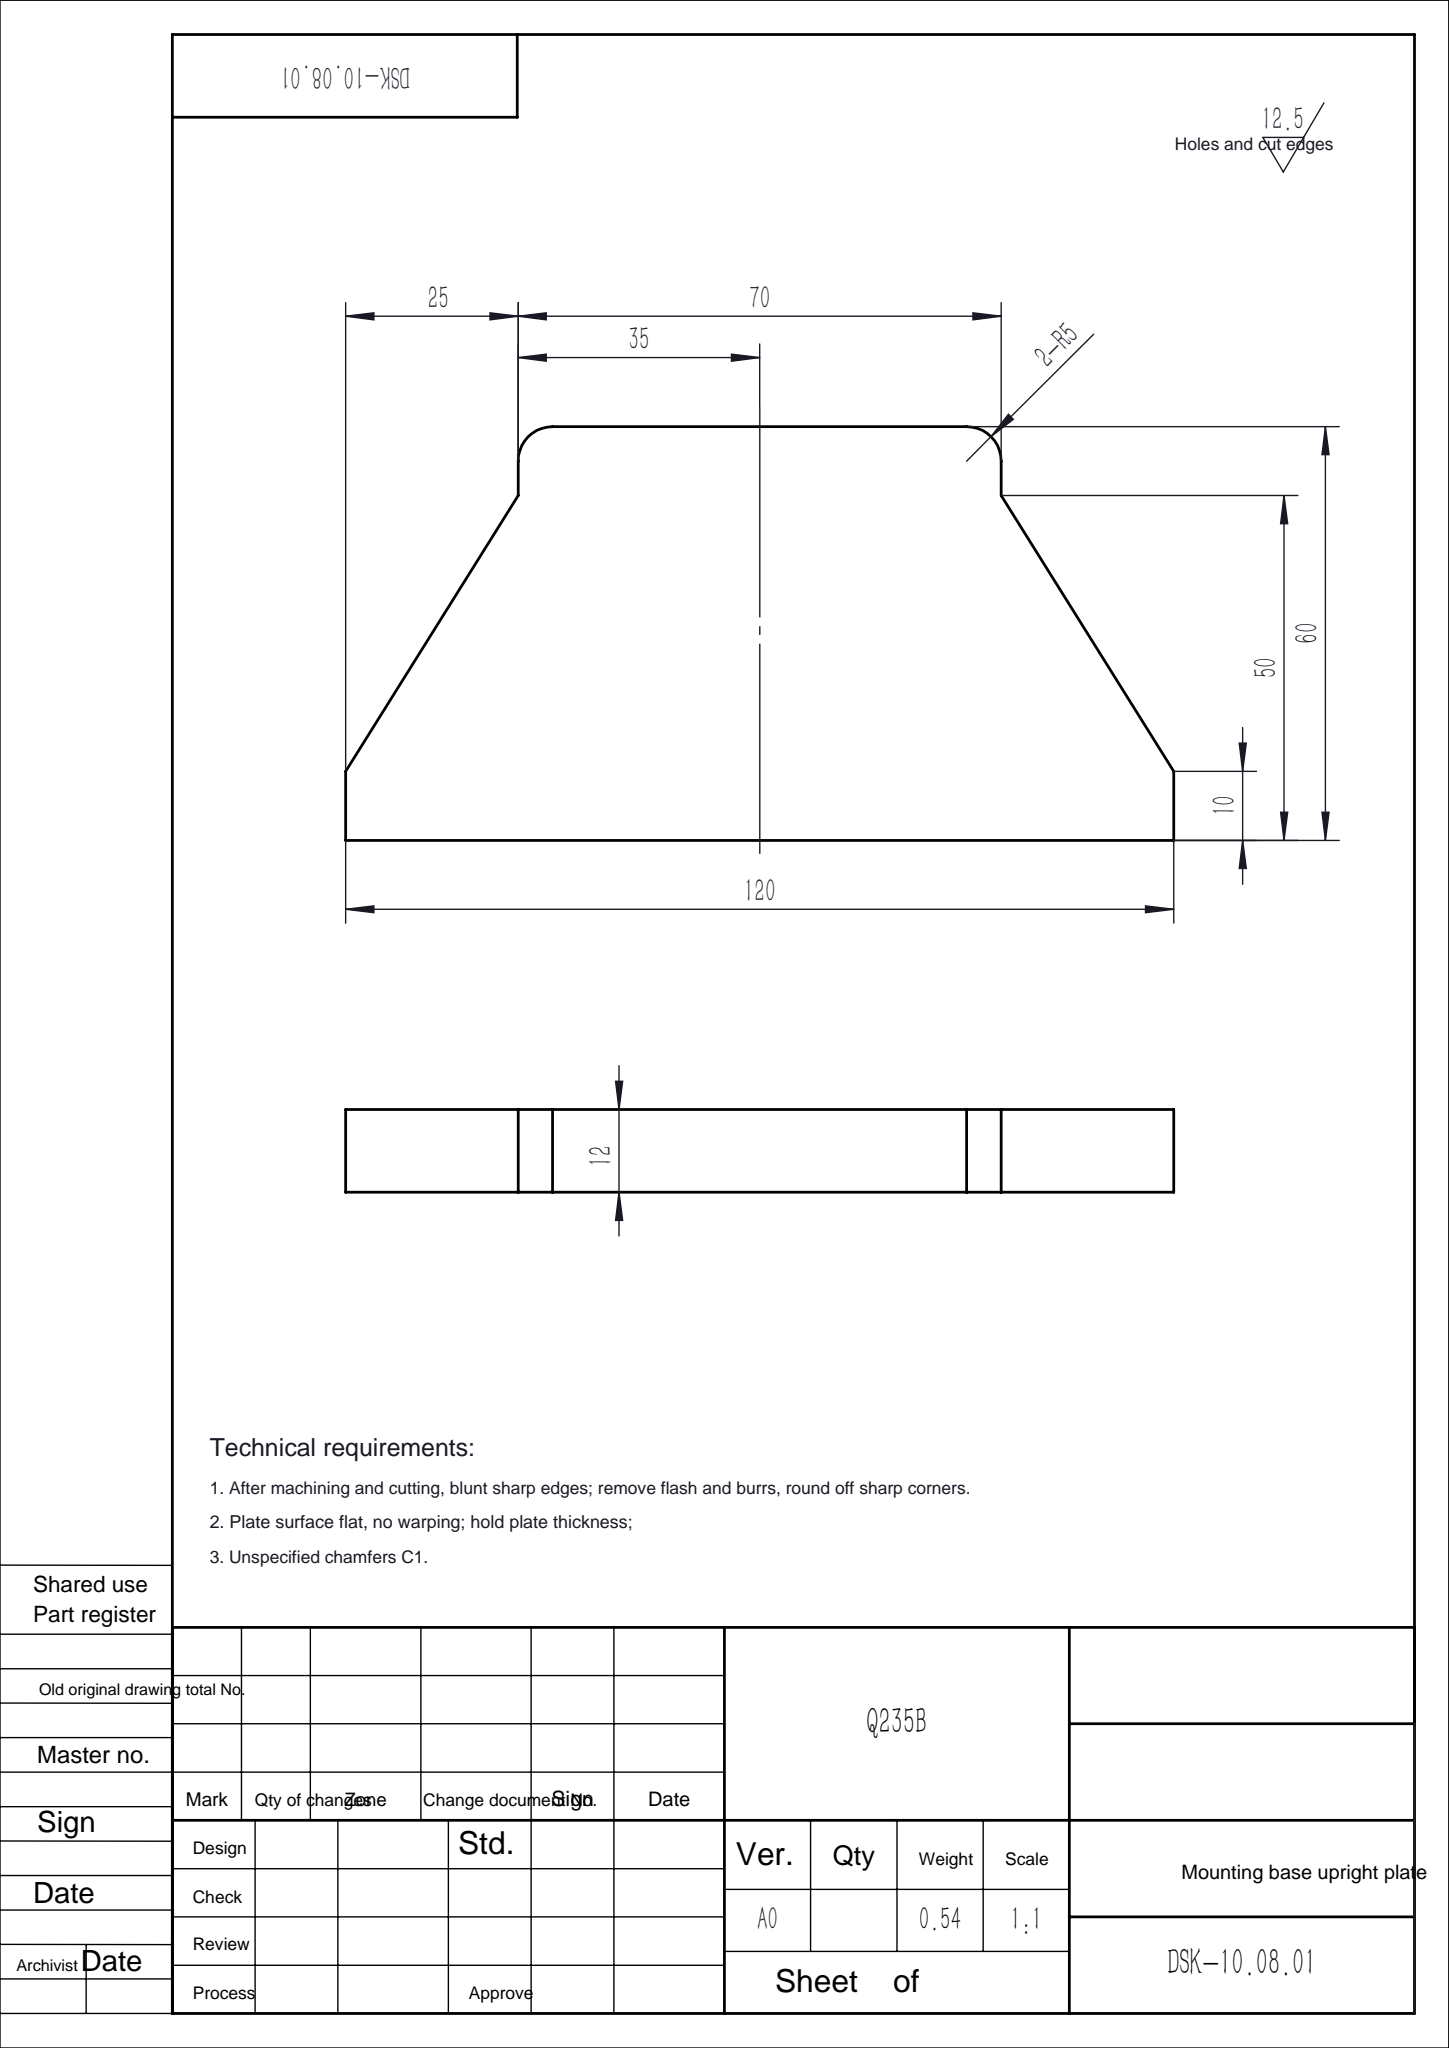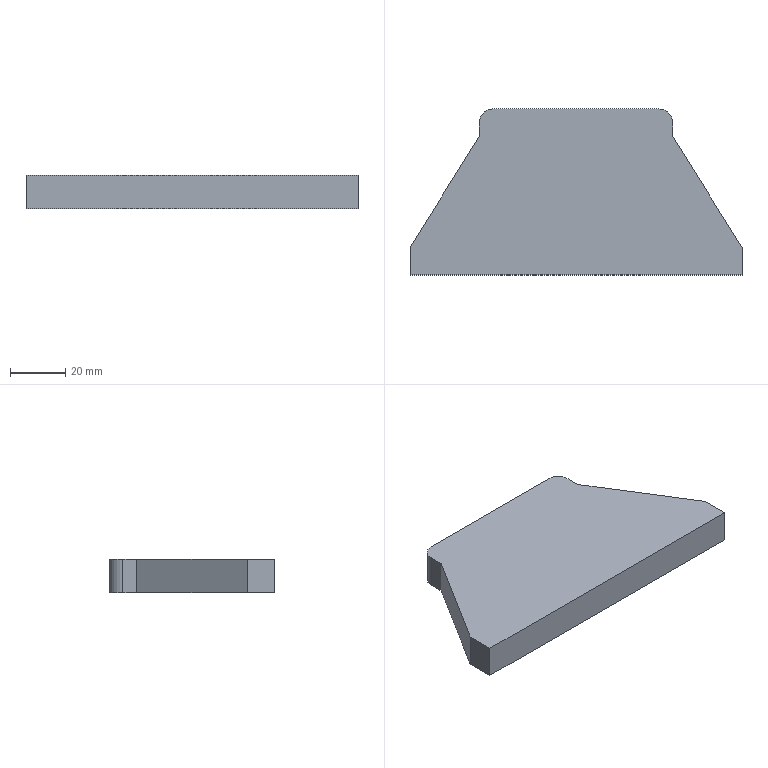Part | SolidWorks | features Extrusion 1, Fillet 1 | 1 solid | 12 faces | box 120 x 60 x 12 mm | volume 68271 mm3 | plane 10 | cylinder 2 | commonest cylinder face diameters 10 x2
STEP:
#1=CARTESIAN_POINT('',(60.,0.,-6.));
#2=VERTEX_POINT('',#1);
#3=CARTESIAN_POINT('',(60.,10.,-6.));
#4=VERTEX_POINT('',#3);
#5=CARTESIAN_POINT('',(60.,0.,-6.));
#6=DIRECTION('',(0.,1.,0.));
#7=VECTOR('',#6,1000.);
#8=LINE('',#5,#7);
#9=EDGE_CURVE('',#2,#4,#8,.T.);
#10=ORIENTED_EDGE('',*,*,#9,.T.);
#11=CARTESIAN_POINT('',(60.,10.,6.));
#12=VERTEX_POINT('',#11);
#13=CARTESIAN_POINT('',(60.,10.,6.));
#14=DIRECTION('',(0.,0.,-1.));
#15=VECTOR('',#14,1000.);
#16=LINE('',#13,#15);
#17=EDGE_CURVE('',#12,#4,#16,.T.);
#18=ORIENTED_EDGE('',*,*,#17,.F.);
#19=CARTESIAN_POINT('',(60.,0.,6.));
#20=VERTEX_POINT('',#19);
#21=CARTESIAN_POINT('',(60.,0.,6.));
#22=DIRECTION('',(0.,1.,0.));
#23=VECTOR('',#22,1000.);
#24=LINE('',#21,#23);
#25=EDGE_CURVE('',#20,#12,#24,.T.);
#26=ORIENTED_EDGE('',*,*,#25,.F.);
#27=CARTESIAN_POINT('',(60.,0.,6.));
#28=DIRECTION('',(0.,0.,-1.));
#29=VECTOR('',#28,1000.);
#30=LINE('',#27,#29);
#31=EDGE_CURVE('',#20,#2,#30,.T.);
#32=ORIENTED_EDGE('',*,*,#31,.T.);
#33=EDGE_LOOP('',(#10,#18,#26,#32));
#34=FACE_OUTER_BOUND('',#33,.T.);
#35=CARTESIAN_POINT('',(60.,0.,6.));
#36=DIRECTION('',(-1.,0.,0.));
#37=DIRECTION('',(0.,0.,1.));
#38=AXIS2_PLACEMENT_3D('',#35,#36,#37);
#39=PLANE('',#38);
#40=ADVANCED_FACE('',(#34),#39,.F.);
#41=CARTESIAN_POINT('',(35.,50.,-6.));
#42=VERTEX_POINT('',#41);
#43=CARTESIAN_POINT('',(60.,10.,-6.));
#44=DIRECTION('',(-0.53,0.848,0.));
#45=VECTOR('',#44,1000.);
#46=LINE('',#43,#45);
#47=EDGE_CURVE('',#4,#42,#46,.T.);
#48=ORIENTED_EDGE('',*,*,#47,.T.);
#49=CARTESIAN_POINT('',(35.,50.,6.));
#50=VERTEX_POINT('',#49);
#51=CARTESIAN_POINT('',(35.,50.,6.));
#52=DIRECTION('',(0.,0.,-1.));
#53=VECTOR('',#52,1000.);
#54=LINE('',#51,#53);
#55=EDGE_CURVE('',#50,#42,#54,.T.);
#56=ORIENTED_EDGE('',*,*,#55,.F.);
#57=CARTESIAN_POINT('',(60.,10.,6.));
#58=DIRECTION('',(-0.53,0.848,0.));
#59=VECTOR('',#58,1000.);
#60=LINE('',#57,#59);
#61=EDGE_CURVE('',#12,#50,#60,.T.);
#62=ORIENTED_EDGE('',*,*,#61,.F.);
#63=ORIENTED_EDGE('',*,*,#17,.T.);
#64=EDGE_LOOP('',(#48,#56,#62,#63));
#65=FACE_OUTER_BOUND('',#64,.T.);
#66=CARTESIAN_POINT('',(60.,10.,6.));
#67=DIRECTION('',(-0.848,-0.53,0.));
#68=DIRECTION('',(0.53,-0.848,0.));
#69=AXIS2_PLACEMENT_3D('',#66,#67,#68);
#70=PLANE('',#69);
#71=ADVANCED_FACE('',(#65),#70,.F.);
#72=CARTESIAN_POINT('',(35.,55.,-6.));
#73=VERTEX_POINT('',#72);
#74=CARTESIAN_POINT('',(35.,50.,-6.));
#75=DIRECTION('',(0.,1.,0.));
#76=VECTOR('',#75,1000.);
#77=LINE('',#74,#76);
#78=EDGE_CURVE('',#42,#73,#77,.T.);
#79=ORIENTED_EDGE('',*,*,#78,.T.);
#80=CARTESIAN_POINT('',(35.,55.,6.));
#81=VERTEX_POINT('',#80);
#82=CARTESIAN_POINT('',(35.,55.,6.));
#83=DIRECTION('',(0.,0.,1.));
#84=VECTOR('',#83,1000.);
#85=LINE('',#82,#84);
#86=EDGE_CURVE('',#73,#81,#85,.T.);
#87=ORIENTED_EDGE('',*,*,#86,.T.);
#88=CARTESIAN_POINT('',(35.,50.,6.));
#89=DIRECTION('',(0.,1.,0.));
#90=VECTOR('',#89,1000.);
#91=LINE('',#88,#90);
#92=EDGE_CURVE('',#50,#81,#91,.T.);
#93=ORIENTED_EDGE('',*,*,#92,.F.);
#94=ORIENTED_EDGE('',*,*,#55,.T.);
#95=EDGE_LOOP('',(#79,#87,#93,#94));
#96=FACE_OUTER_BOUND('',#95,.T.);
#97=CARTESIAN_POINT('',(35.,50.,6.));
#98=DIRECTION('',(-1.,0.,0.));
#99=DIRECTION('',(0.,0.,1.));
#100=AXIS2_PLACEMENT_3D('',#97,#98,#99);
#101=PLANE('',#100);
#102=ADVANCED_FACE('',(#96),#101,.F.);
#103=CARTESIAN_POINT('',(30.,60.,6.));
#104=VERTEX_POINT('',#103);
#105=CARTESIAN_POINT('',(-30.,60.,6.));
#106=VERTEX_POINT('',#105);
#107=CARTESIAN_POINT('',(35.,60.,6.));
#108=DIRECTION('',(-1.,0.,0.));
#109=VECTOR('',#108,1000.);
#110=LINE('',#107,#109);
#111=EDGE_CURVE('',#104,#106,#110,.T.);
#112=ORIENTED_EDGE('',*,*,#111,.F.);
#113=CARTESIAN_POINT('',(30.,60.,-6.));
#114=VERTEX_POINT('',#113);
#115=CARTESIAN_POINT('',(30.,60.,6.));
#116=DIRECTION('',(0.,0.,-1.));
#117=VECTOR('',#116,1000.);
#118=LINE('',#115,#117);
#119=EDGE_CURVE('',#104,#114,#118,.T.);
#120=ORIENTED_EDGE('',*,*,#119,.T.);
#121=CARTESIAN_POINT('',(-30.,60.,-6.));
#122=VERTEX_POINT('',#121);
#123=CARTESIAN_POINT('',(35.,60.,-6.));
#124=DIRECTION('',(-1.,0.,0.));
#125=VECTOR('',#124,1000.);
#126=LINE('',#123,#125);
#127=EDGE_CURVE('',#114,#122,#126,.T.);
#128=ORIENTED_EDGE('',*,*,#127,.T.);
#129=CARTESIAN_POINT('',(-30.,60.,6.));
#130=DIRECTION('',(0.,0.,1.));
#131=VECTOR('',#130,1000.);
#132=LINE('',#129,#131);
#133=EDGE_CURVE('',#122,#106,#132,.T.);
#134=ORIENTED_EDGE('',*,*,#133,.T.);
#135=EDGE_LOOP('',(#112,#120,#128,#134));
#136=FACE_OUTER_BOUND('',#135,.T.);
#137=CARTESIAN_POINT('',(35.,60.,6.));
#138=DIRECTION('',(0.,-1.,0.));
#139=DIRECTION('',(1.,0.,0.));
#140=AXIS2_PLACEMENT_3D('',#137,#138,#139);
#141=PLANE('',#140);
#142=ADVANCED_FACE('',(#136),#141,.F.);
#143=CARTESIAN_POINT('',(-35.,55.,6.));
#144=VERTEX_POINT('',#143);
#145=CARTESIAN_POINT('',(-35.,50.,6.));
#146=VERTEX_POINT('',#145);
#147=CARTESIAN_POINT('',(-35.,50.,6.));
#148=DIRECTION('',(0.,-1.,0.));
#149=VECTOR('',#148,1000.);
#150=LINE('',#147,#149);
#151=EDGE_CURVE('',#144,#146,#150,.T.);
#152=ORIENTED_EDGE('',*,*,#151,.F.);
#153=CARTESIAN_POINT('',(-35.,55.,-6.));
#154=VERTEX_POINT('',#153);
#155=CARTESIAN_POINT('',(-35.,55.,6.));
#156=DIRECTION('',(0.,0.,-1.));
#157=VECTOR('',#156,1000.);
#158=LINE('',#155,#157);
#159=EDGE_CURVE('',#144,#154,#158,.T.);
#160=ORIENTED_EDGE('',*,*,#159,.T.);
#161=CARTESIAN_POINT('',(-35.,50.,-6.));
#162=VERTEX_POINT('',#161);
#163=CARTESIAN_POINT('',(-35.,50.,-6.));
#164=DIRECTION('',(0.,-1.,0.));
#165=VECTOR('',#164,1000.);
#166=LINE('',#163,#165);
#167=EDGE_CURVE('',#154,#162,#166,.T.);
#168=ORIENTED_EDGE('',*,*,#167,.T.);
#169=CARTESIAN_POINT('',(-35.,50.,6.));
#170=DIRECTION('',(0.,0.,-1.));
#171=VECTOR('',#170,1000.);
#172=LINE('',#169,#171);
#173=EDGE_CURVE('',#146,#162,#172,.T.);
#174=ORIENTED_EDGE('',*,*,#173,.F.);
#175=EDGE_LOOP('',(#152,#160,#168,#174));
#176=FACE_OUTER_BOUND('',#175,.T.);
#177=CARTESIAN_POINT('',(-35.,50.,6.));
#178=DIRECTION('',(1.,0.,0.));
#179=DIRECTION('',(0.,0.,-1.));
#180=AXIS2_PLACEMENT_3D('',#177,#178,#179);
#181=PLANE('',#180);
#182=ADVANCED_FACE('',(#176),#181,.F.);
#183=CARTESIAN_POINT('',(-60.,10.,-6.));
#184=VERTEX_POINT('',#183);
#185=CARTESIAN_POINT('',(-60.,10.,-6.));
#186=DIRECTION('',(-0.53,-0.848,0.));
#187=VECTOR('',#186,1000.);
#188=LINE('',#185,#187);
#189=EDGE_CURVE('',#162,#184,#188,.T.);
#190=ORIENTED_EDGE('',*,*,#189,.T.);
#191=CARTESIAN_POINT('',(-60.,10.,6.));
#192=VERTEX_POINT('',#191);
#193=CARTESIAN_POINT('',(-60.,10.,6.));
#194=DIRECTION('',(0.,0.,-1.));
#195=VECTOR('',#194,1000.);
#196=LINE('',#193,#195);
#197=EDGE_CURVE('',#192,#184,#196,.T.);
#198=ORIENTED_EDGE('',*,*,#197,.F.);
#199=CARTESIAN_POINT('',(-60.,10.,6.));
#200=DIRECTION('',(-0.53,-0.848,0.));
#201=VECTOR('',#200,1000.);
#202=LINE('',#199,#201);
#203=EDGE_CURVE('',#146,#192,#202,.T.);
#204=ORIENTED_EDGE('',*,*,#203,.F.);
#205=ORIENTED_EDGE('',*,*,#173,.T.);
#206=EDGE_LOOP('',(#190,#198,#204,#205));
#207=FACE_OUTER_BOUND('',#206,.T.);
#208=CARTESIAN_POINT('',(-60.,10.,6.));
#209=DIRECTION('',(0.848,-0.53,0.));
#210=DIRECTION('',(0.53,0.848,0.));
#211=AXIS2_PLACEMENT_3D('',#208,#209,#210);
#212=PLANE('',#211);
#213=ADVANCED_FACE('',(#207),#212,.F.);
#214=CARTESIAN_POINT('',(-60.,0.,-6.));
#215=VERTEX_POINT('',#214);
#216=CARTESIAN_POINT('',(-60.,0.,-6.));
#217=DIRECTION('',(0.,-1.,0.));
#218=VECTOR('',#217,1000.);
#219=LINE('',#216,#218);
#220=EDGE_CURVE('',#184,#215,#219,.T.);
#221=ORIENTED_EDGE('',*,*,#220,.T.);
#222=CARTESIAN_POINT('',(-60.,0.,6.));
#223=VERTEX_POINT('',#222);
#224=CARTESIAN_POINT('',(-60.,0.,6.));
#225=DIRECTION('',(0.,0.,-1.));
#226=VECTOR('',#225,1000.);
#227=LINE('',#224,#226);
#228=EDGE_CURVE('',#223,#215,#227,.T.);
#229=ORIENTED_EDGE('',*,*,#228,.F.);
#230=CARTESIAN_POINT('',(-60.,0.,6.));
#231=DIRECTION('',(0.,-1.,0.));
#232=VECTOR('',#231,1000.);
#233=LINE('',#230,#232);
#234=EDGE_CURVE('',#192,#223,#233,.T.);
#235=ORIENTED_EDGE('',*,*,#234,.F.);
#236=ORIENTED_EDGE('',*,*,#197,.T.);
#237=EDGE_LOOP('',(#221,#229,#235,#236));
#238=FACE_OUTER_BOUND('',#237,.T.);
#239=CARTESIAN_POINT('',(-60.,0.,6.));
#240=DIRECTION('',(1.,0.,0.));
#241=DIRECTION('',(0.,1.,0.));
#242=AXIS2_PLACEMENT_3D('',#239,#240,#241);
#243=PLANE('',#242);
#244=ADVANCED_FACE('',(#238),#243,.F.);
#245=CARTESIAN_POINT('',(-60.,0.,-6.));
#246=DIRECTION('',(1.,0.,0.));
#247=VECTOR('',#246,1000.);
#248=LINE('',#245,#247);
#249=EDGE_CURVE('',#215,#2,#248,.T.);
#250=ORIENTED_EDGE('',*,*,#249,.T.);
#251=ORIENTED_EDGE('',*,*,#31,.F.);
#252=CARTESIAN_POINT('',(-60.,0.,6.));
#253=DIRECTION('',(1.,0.,0.));
#254=VECTOR('',#253,1000.);
#255=LINE('',#252,#254);
#256=EDGE_CURVE('',#223,#20,#255,.T.);
#257=ORIENTED_EDGE('',*,*,#256,.F.);
#258=ORIENTED_EDGE('',*,*,#228,.T.);
#259=EDGE_LOOP('',(#250,#251,#257,#258));
#260=FACE_OUTER_BOUND('',#259,.T.);
#261=CARTESIAN_POINT('',(-60.,0.,6.));
#262=DIRECTION('',(0.,1.,0.));
#263=DIRECTION('',(0.,0.,1.));
#264=AXIS2_PLACEMENT_3D('',#261,#262,#263);
#265=PLANE('',#264);
#266=ADVANCED_FACE('',(#260),#265,.F.);
#267=ORIENTED_EDGE('',*,*,#92,.T.);
#268=CARTESIAN_POINT('',(30.,55.,6.));
#269=DIRECTION('',(0.,0.,1.));
#270=DIRECTION('',(1.,0.,0.));
#271=AXIS2_PLACEMENT_3D('',#268,#269,#270);
#272=CIRCLE('',#271,5.);
#273=EDGE_CURVE('',#81,#104,#272,.T.);
#274=ORIENTED_EDGE('',*,*,#273,.T.);
#275=ORIENTED_EDGE('',*,*,#111,.T.);
#276=CARTESIAN_POINT('',(-30.,55.,6.));
#277=DIRECTION('',(0.,0.,1.));
#278=DIRECTION('',(1.,0.,0.));
#279=AXIS2_PLACEMENT_3D('',#276,#277,#278);
#280=CIRCLE('',#279,5.);
#281=EDGE_CURVE('',#106,#144,#280,.T.);
#282=ORIENTED_EDGE('',*,*,#281,.T.);
#283=ORIENTED_EDGE('',*,*,#151,.T.);
#284=ORIENTED_EDGE('',*,*,#203,.T.);
#285=ORIENTED_EDGE('',*,*,#234,.T.);
#286=ORIENTED_EDGE('',*,*,#256,.T.);
#287=ORIENTED_EDGE('',*,*,#25,.T.);
#288=ORIENTED_EDGE('',*,*,#61,.T.);
#289=EDGE_LOOP('',(#267,#274,#275,#282,#283,#284,#285,#286,#287,#288));
#290=FACE_OUTER_BOUND('',#289,.T.);
#291=CARTESIAN_POINT('',(0.,0.,6.));
#292=DIRECTION('',(0.,0.,1.));
#293=DIRECTION('',(1.,0.,0.));
#294=AXIS2_PLACEMENT_3D('',#291,#292,#293);
#295=PLANE('',#294);
#296=ADVANCED_FACE('',(#290),#295,.T.);
#297=ORIENTED_EDGE('',*,*,#127,.F.);
#298=CARTESIAN_POINT('',(30.,55.,-6.));
#299=DIRECTION('',(0.,0.,-1.));
#300=DIRECTION('',(1.,0.,0.));
#301=AXIS2_PLACEMENT_3D('',#298,#299,#300);
#302=CIRCLE('',#301,5.);
#303=EDGE_CURVE('',#114,#73,#302,.T.);
#304=ORIENTED_EDGE('',*,*,#303,.T.);
#305=ORIENTED_EDGE('',*,*,#78,.F.);
#306=ORIENTED_EDGE('',*,*,#47,.F.);
#307=ORIENTED_EDGE('',*,*,#9,.F.);
#308=ORIENTED_EDGE('',*,*,#249,.F.);
#309=ORIENTED_EDGE('',*,*,#220,.F.);
#310=ORIENTED_EDGE('',*,*,#189,.F.);
#311=ORIENTED_EDGE('',*,*,#167,.F.);
#312=CARTESIAN_POINT('',(-30.,55.,-6.));
#313=DIRECTION('',(0.,0.,-1.));
#314=DIRECTION('',(1.,0.,0.));
#315=AXIS2_PLACEMENT_3D('',#312,#313,#314);
#316=CIRCLE('',#315,5.);
#317=EDGE_CURVE('',#154,#122,#316,.T.);
#318=ORIENTED_EDGE('',*,*,#317,.T.);
#319=EDGE_LOOP('',(#297,#304,#305,#306,#307,#308,#309,#310,#311,#318));
#320=FACE_OUTER_BOUND('',#319,.T.);
#321=CARTESIAN_POINT('',(0.,0.,-6.));
#322=DIRECTION('',(0.,0.,1.));
#323=DIRECTION('',(1.,0.,0.));
#324=AXIS2_PLACEMENT_3D('',#321,#322,#323);
#325=PLANE('',#324);
#326=ADVANCED_FACE('',(#320),#325,.F.);
#327=ORIENTED_EDGE('',*,*,#273,.F.);
#328=ORIENTED_EDGE('',*,*,#86,.F.);
#329=ORIENTED_EDGE('',*,*,#303,.F.);
#330=ORIENTED_EDGE('',*,*,#119,.F.);
#331=EDGE_LOOP('',(#327,#328,#329,#330));
#332=FACE_OUTER_BOUND('',#331,.T.);
#333=CARTESIAN_POINT('',(30.,55.,6.));
#334=DIRECTION('',(0.,0.,-1.));
#335=DIRECTION('',(-1.,0.,0.));
#336=AXIS2_PLACEMENT_3D('',#333,#334,#335);
#337=CYLINDRICAL_SURFACE('',#336,5.);
#338=ADVANCED_FACE('',(#332),#337,.T.);
#339=ORIENTED_EDGE('',*,*,#281,.F.);
#340=ORIENTED_EDGE('',*,*,#133,.F.);
#341=ORIENTED_EDGE('',*,*,#317,.F.);
#342=ORIENTED_EDGE('',*,*,#159,.F.);
#343=EDGE_LOOP('',(#339,#340,#341,#342));
#344=FACE_OUTER_BOUND('',#343,.T.);
#345=CARTESIAN_POINT('',(-30.,55.,6.));
#346=DIRECTION('',(0.,0.,-1.));
#347=DIRECTION('',(-1.,0.,0.));
#348=AXIS2_PLACEMENT_3D('',#345,#346,#347);
#349=CYLINDRICAL_SURFACE('',#348,5.);
#350=ADVANCED_FACE('',(#344),#349,.T.);
#351=CLOSED_SHELL('',(#40,#71,#102,#142,#182,#213,#244,#266,#296,#326,#338,#350));
#352=MANIFOLD_SOLID_BREP('',#351);
#353=CARTESIAN_POINT('',(0.,0.,0.));
#354=DIRECTION('',(0.,0.,1.));
#355=DIRECTION('',(1.,0.,0.));
#356=AXIS2_PLACEMENT_3D('',#353,#354,#355);
#357=(LENGTH_UNIT()NAMED_UNIT(*)SI_UNIT(.MILLI.,.METRE.));
#358=UNCERTAINTY_MEASURE_WITH_UNIT(LENGTH_MEASURE(0.00001),#357,'','');
#359=(NAMED_UNIT(*)PLANE_ANGLE_UNIT()SI_UNIT($,.RADIAN.));
#360=(NAMED_UNIT(*)SI_UNIT($,.STERADIAN.)SOLID_ANGLE_UNIT());
#361=(GEOMETRIC_REPRESENTATION_CONTEXT(3)GLOBAL_UNCERTAINTY_ASSIGNED_CONTEXT((#358))GLOBAL_UNIT_ASSIGNED_CONTEXT((#357,#359,#360))REPRESENTATION_CONTEXT('',''));
#362=ADVANCED_BREP_SHAPE_REPRESENTATION('',(#352,#356),#361);